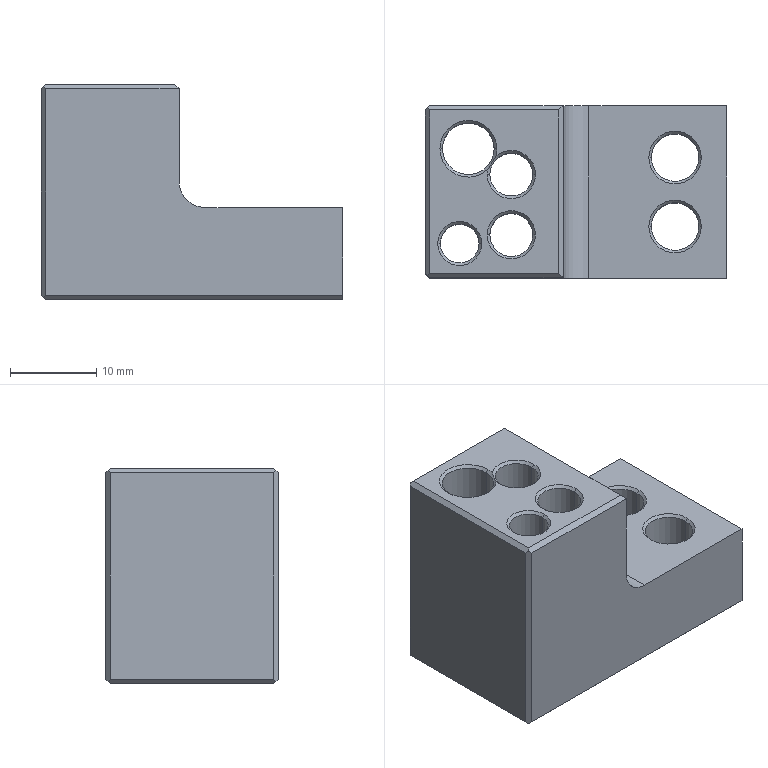Part | NX | 1 solid | 54 faces | box 35 x 20 x 25 mm | volume 9475 mm3 | cone 24 | plane 17 | cylinder 13 | commonest cylinder face diameters 5 x4 5.5 x4 6 x3 4.5 x2